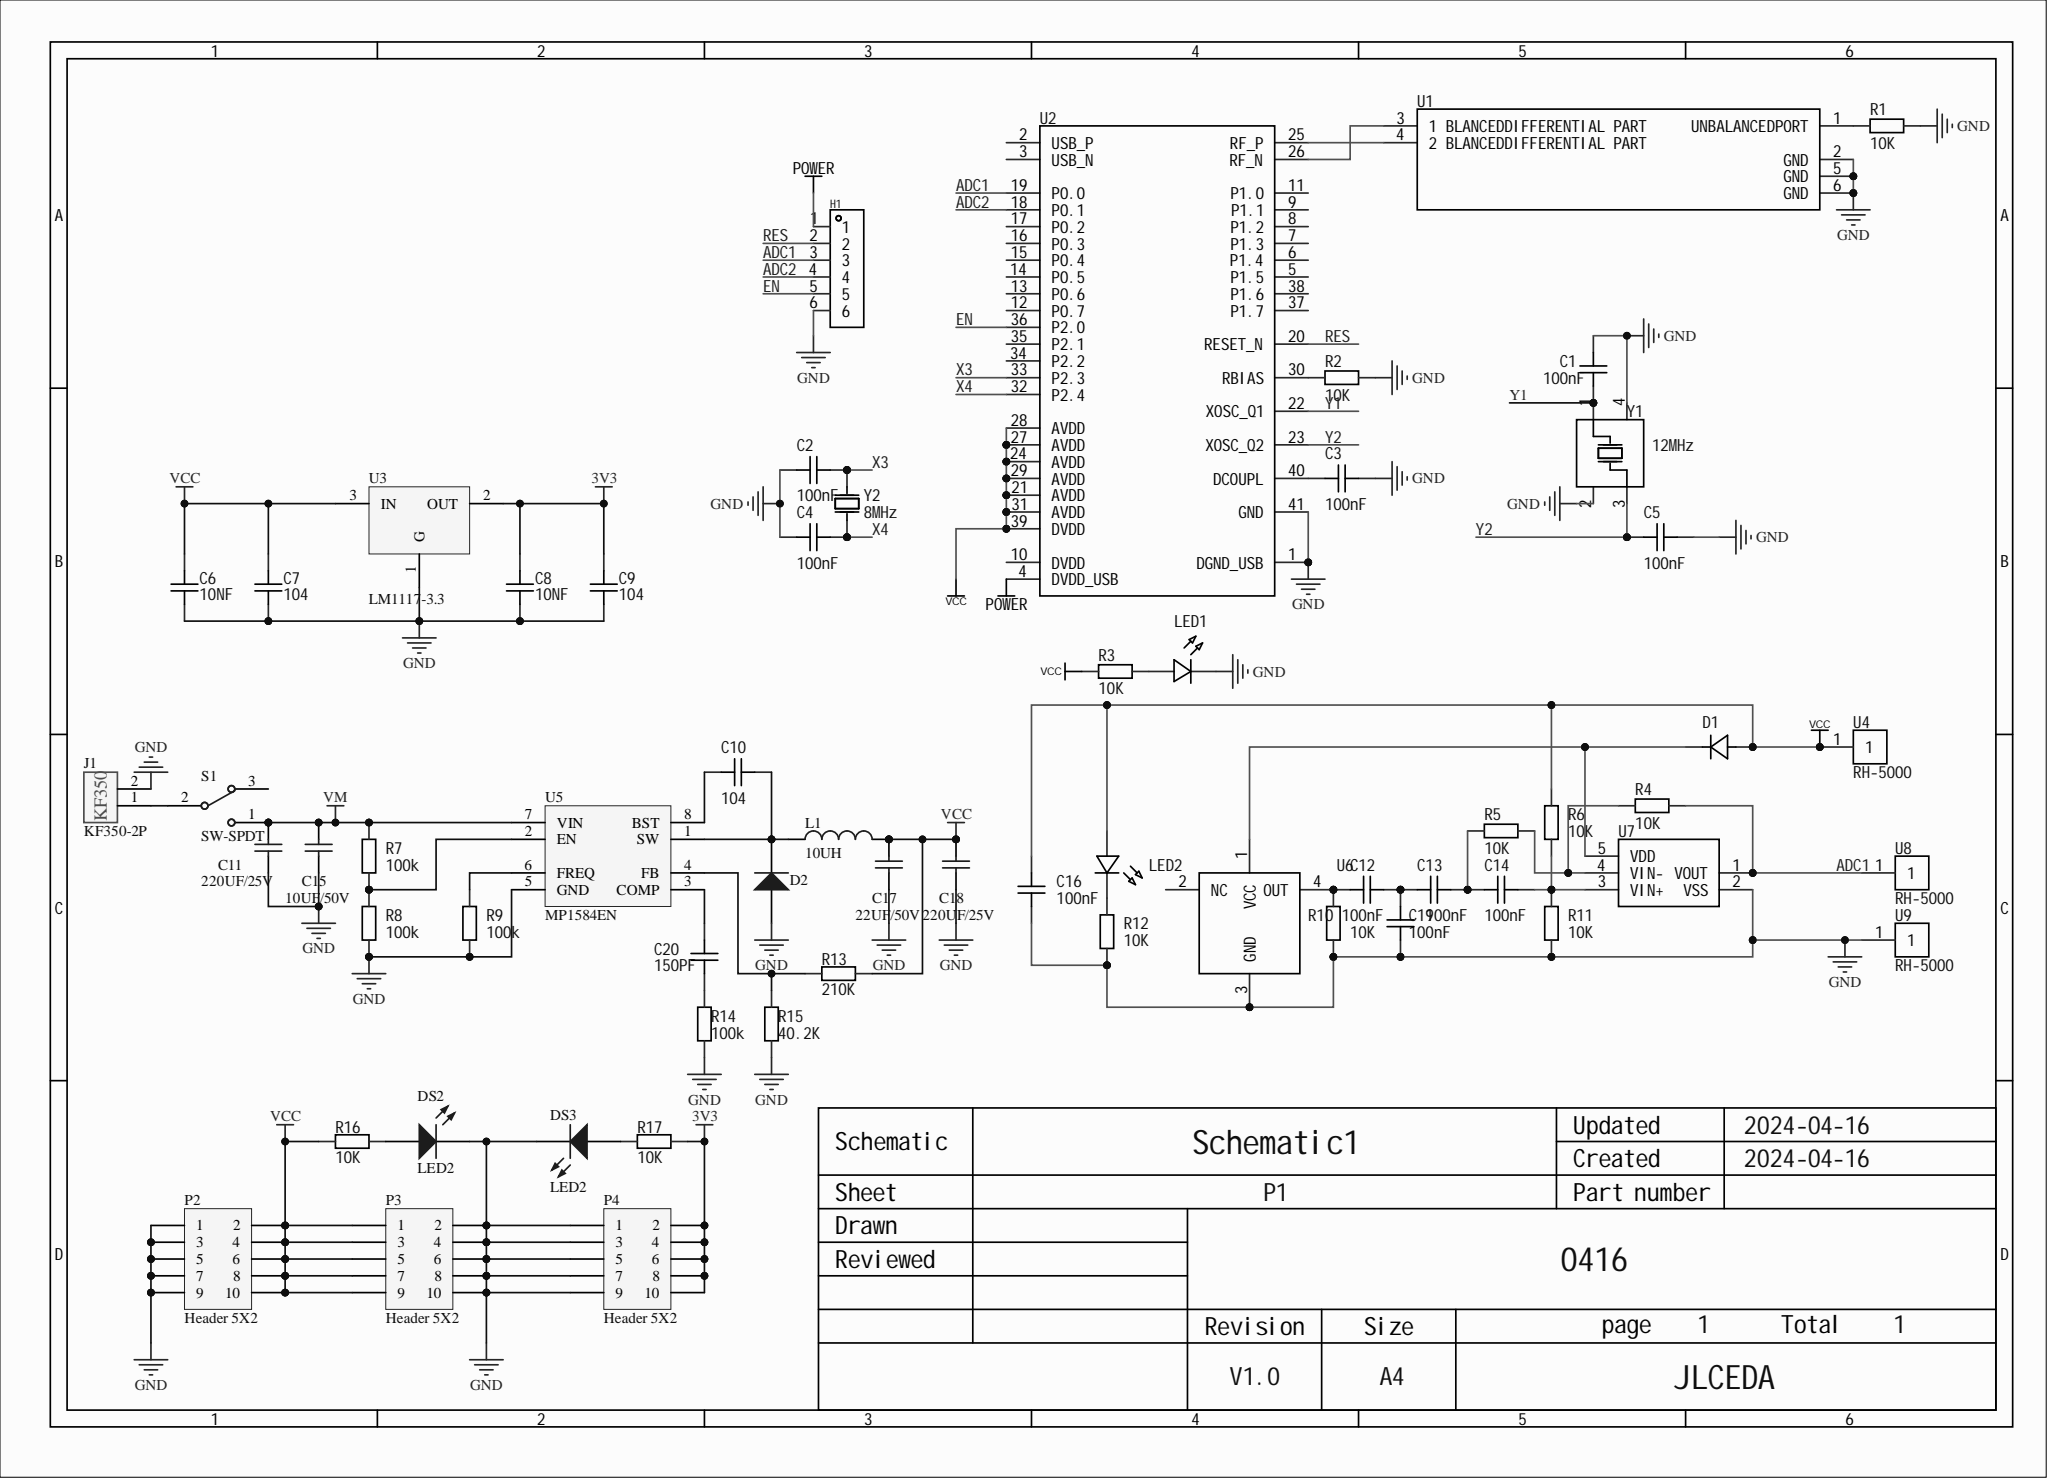Circuit board | Altium Designer | 61 parts | 36 nets
Bill of materials:
Comment,Description,Designator,Footprint,LibRef,Quantity
"100nF","","C1, C2, C3, C4, C5, C6, C7, C8, C9, C10, C12, C13, C14, C16, C19, C20","C0603","CAP_0603","16"
"220UF/25V","Capacitor (Semiconductor SIM Model)","C11, C18","贴片电容","Cap Semi","2"
"10UF/50V","Capacitor (Semiconductor SIM Model)","C15","贴片电容","Cap Semi","1"
"22UF/50V","Capacitor (Semiconductor SIM Model)","C17","贴片电容","Cap Semi","1"
"D_1N4007A","","D1","3.2X1.6X1.1","D_1N4007A","1"
"Diode BAS16","Silicon Switching Diode for High-Speed Switching","D2","3.2X1.6X1.1","Diode BAS16","1"
"LED2","Typical RED, GREEN, YELLOW, AMBER GaAs LED","DS2, DS3","my0603LED","LED2","2"
"HDR-F_2.54_1x6P","","H1","HDR1X6","HDR-F_2.54_1x6P","1"
"KF350-2P","","J1","KF350-2P","KF350-2P","1"
"10UH","Inductor","L1","0402-A","Inductor","1"
"LED_0603-R","","LED1, LED2","my0603LED","LED_0603-R","2"
"Header 5X2","Header, 5-Pin, Dual row","P2, P3, P4","HDR2X5","Header 5X2","3"
"10K","","R1, R2, R3, R4, R5, R6, R7, R8, R9, R10, R11, R12, R13, R14, R15, R16, R17","my0603","Res_0603","17"
"SW-SPDT","SPDT Subminiature Toggle Switch, Right Angle Mounting, Vertical Actuation","S1","TL36WW15050","SW-SPDT","1"
"BL1","","U1","TSOP-6 - duplicate","BL1","1"
"CC2540","","U2","CC254X_QFN","CC2540","1"
"LM1117-3.3","LINER REG","U3","LM1117-3.3","LM1117","1"
"RH-5000","","U4, U8, U9","TEST-TH_BD2.54-P1.4_RED","RH-5000","3"
"MP1584EN","","U5","MP1548EN","MP1584EN","1"
"APDS","","U6","SENSORS-SMD_APDS-9008-020","APDS","1"
"AMP","","U7","MCP6001","AMP","1"
"12MHz","Crystal type: SMD crystal; frequency: 12MHz; frequency tolerance (room temp): ±10ppm; load capacitance: 20pF; frequency stability (full temp): ±20ppm;","Y1","OSC-SMD_4P-L5.0-W3.2-BL","X322512MSB4SI","1"
"8MHz","Crystal type: SMD crystal; frequency: 8MHz; frequency tolerance (room temp): ±20ppm; load capacitance: 20pF; frequency stability (full temp): ±30ppm;","Y2","XTAL_US","X49SM8MSD2SC","1"
Netlist (Protel format):
[
C1
C0603
100nF



]
[
C2
C0603
100nF



]
[
C3
C0603
100nF



]
[
C4
C0603
100nF



]
[
C5
C0603
100nF



]
[
C6
C0603
100nF



]
[
C7
C0603
100nF



]
[
C8
C0603
100nF



]
[
C9
C0603
100nF



]
[
C10
C0603
100nF



]
[
C11
贴片电容
220UF/25V



]
[
C12
C0603
100nF



]
[
C13
C0603
100nF



]
[
C14
C0603
100nF



]
[
C15
贴片电容
10UF/50V



]
[
C16
C0603
100nF



]
[
C17
贴片电容
22UF/50V



]
[
C18
贴片电容
220UF/25V



]
[
C19
C0603
100nF



]
[
C20
C0603
100nF



]
[
D1
3.2X1.6X1.1
D_1N4007A



]
[
D2
3.2X1.6X1.1
Diode BAS16



]
[
DS2
my0603LED
LED2



]
[
DS3
my0603LED
LED2



]
[
H1
HDR1X6
HDR-F_2.54_1x6P



]
[
J1
KF350-2P
KF350-2P



]
[
L1
0402-A
10UH



]
[
LED1
my0603LED
LED_0603-R



]
[
LED2
my0603LED
LED_0603-R



]
[
P2
HDR2X5
Header 5X2



]
[
P3
HDR2X5
Header 5X2



]
[
P4
HDR2X5
Header 5X2



]
[
R1
my0603
10K



]
[
R2
my0603
10K



]
[
R3
my0603
10K



]
[
R4
my0603
10K



]
[
R5
my0603
10K



]
[
R6
my0603
10K



]
[
R7
my0603
10K



]
[
R8
my0603
10K



]
[
R9
my0603
10K



]
[
R10
my0603
10K



]
[
R11
my0603
10K



]
[
R12
my0603
10K



]
[
R13
my0603
10K



]
[
R14
my0603
10K



]
[
R15
my0603
10K



]
[
R16
my0603
10K



]
[
R17
my0603
10K



]
[
S1
TL36WW15050
SW-SPDT



]
[
U1
TSOP-6 - duplicate
BL1



]
[
U2
CC254X_QFN
CC2540



]
[
U3
LM1117-3.3
LM1117-3.3



]
[
U4
TEST-TH_BD2.54-P1.4_RED
RH-5000



]
[
U5
MP1548EN
MP1584EN



]
[
U6
SENSORS-SMD_APDS-9008-020
APDS



]
[
U7
MCP6001
AMP



]
[
U8
TEST-TH_BD2.54-P1.4_RED
RH-5000



]
[
U9
TEST-TH_BD2.54-P1.4_RED
RH-5000



]
[
Y1
OSC-SMD_4P-L5.0-W3.2-BL
12MHz



]
[
Y2
XTAL_US
8MHz



]
(
Y2
C5-2
U2-23
Y1-3
)
(
Y1
C1-2
U2-22
Y1-1
)
(
X4
C4-2
U2-32
Y2-2
)
(
X3
C2-2
U2-33
Y2-1
)
(
VM
C11-2
C15-2
R7-2
S1-1
U5-7
)
(
VCC
C6-2
C7-2
C16-2
C17-2
C18-2
D1-2
L1-2
LED2-2
P2-2
P2-4
P2-6
P2-8
P2-10
P3-1
P3-3
P3-5
P3-7
P3-9
R3-1
R6-2
R13-1
R16-2
U2-21
U2-24
U2-27
U2-28
U2-29
U2-31
U2-39
U3-3
U4-1
)
(
RES
H1-2
U2-20
)
(
POWER
H1-1
U2-4
)
(
NetU1_4
U1-4
U2-25
)
(
NetU1_3
U1-3
U2-26
)
(
NetR13_2
R13-2
R15-1
U5-4
)
(
NetR9_2
R9-2
U5-6
)
(
NetR7_1
R7-1
R8-2
U5-2
)
(
NetR4_2
R4-2
R5-2
U7-4
)
(
NetR2_1
R2-1
U2-30
)
(
NetR1_1
R1-1
U1-1
)
(
NetLED2_1
LED2-1
R12-2
)
(
NetLED1_2
LED1-2
R3-2
)
(
NetJ1_1
J1-1
S1-2
)
(
NetDS3_1
DS3-1
R17-2
)
(
NetDS2_1
DS2-1
R16-1
)
(
NetD1_1
D1-1
U6-1
U7-5
)
(
NetC20_2
C20-2
U5-3
)
(
NetC20_1
C20-1
R14-1
)
(
NetC14_1
C14-1
R6-1
R11-2
U7-3
)
(
NetC13_2
C13-2
C14-2
R5-1
)
(
NetC12_2
C12-2
C13-1
C19-2
)
(
NetC12_1
C12-1
R10-2
U6-4
)
(
NetC10_2
C10-2
D2-3
L1-1
U5-1
)
(
NetC10_1
C10-1
U5-8
)
(
NetC3_1
C3-1
U2-40
)
(
GND
C1-1
C2-1
C3-2
C4-1
C5-1
C6-1
C7-1
C8-1
C9-1
C11-1
C15-1
C16-1
C17-1
C18-1
C19-1
D2-1
DS2-2
DS3-2
H1-6
J1-2
LED1-1
P2-1
P2-3
P2-5
P2-7
P2-9
P3-2
P3-4
P3-6
P3-8
P3-10
P4-1
P4-3
P4-5
P4-7
P4-9
R1-2
R2-2
R8-1
R9-1
R10-1
R11-1
R12-1
R14-2
R15-2
U1-2
U1-5
U1-6
U2-1
U2-41
U3-1
U5-5
U6-3
U7-2
U9-1
Y1-2
Y1-4
)
(
EN
H1-5
U2-36
)
(
ADC2
H1-4
U2-18
)
(
ADC1
H1-3
R4-1
U2-19
U7-1
U8-1
)
(
3V3
C8-2
C9-2
P4-2
P4-4
P4-6
P4-8
P4-10
R17-1
U3-2
)